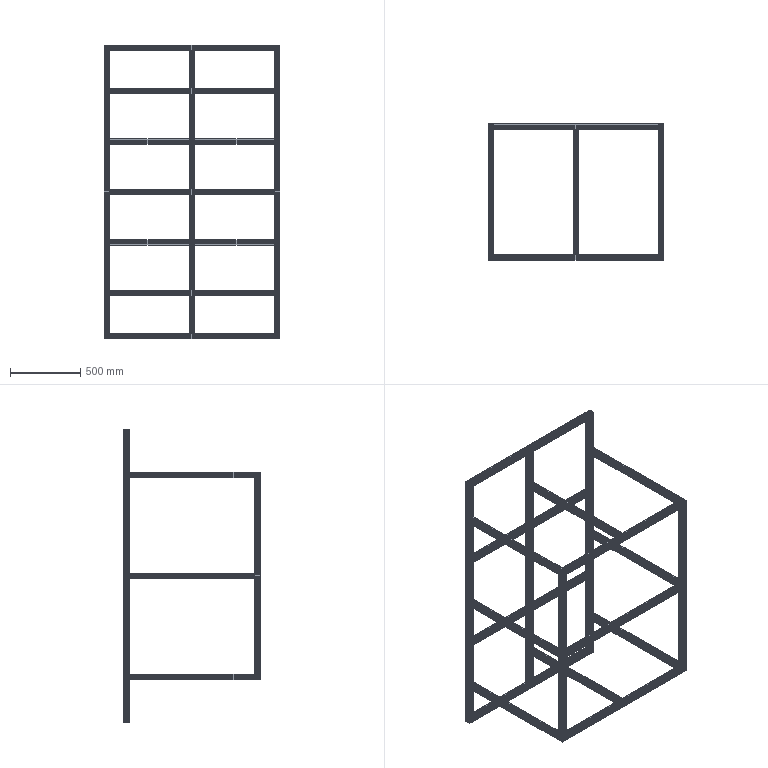Part | SolidWorks | features ICE 8, Extrusion 1 | 22 solids | 2684 faces | box 1250 x 970 x 2090 mm | volume 12416282 mm3 | plane 2068 | cylinder 616 | commonest cylinder face diameters 1 x440 10.2 x176